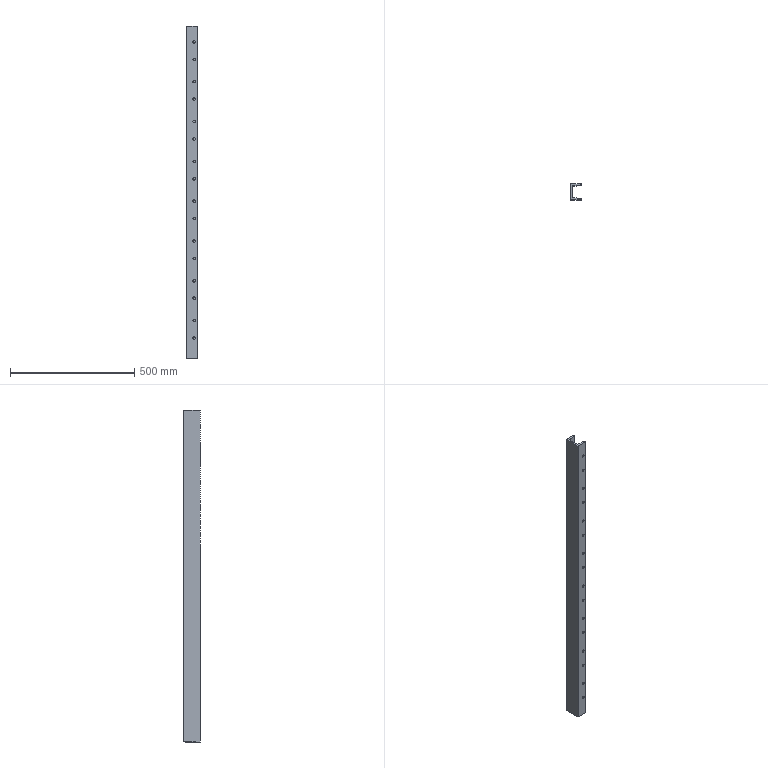Part | STEP file | DIN 1026-1 U 65 1785352380506 | 1 solid | 30 faces | box 42 x 65 x 1334 mm | volume 1196644 mm3 | cylinder 20 | plane 10 | commonest cylinder face diameters 10 x16 8 x2 15 x2
STEP:
#1=CARTESIAN_POINT('',(24.5,-32.5,1200.233));
#2=VERTEX_POINT('',#1);
#3=CARTESIAN_POINT('',(29.5,-32.5,1200.233));
#4=DIRECTION('',(0.,1.,0.));
#5=DIRECTION('',(1.,0.,0.));
#6=AXIS2_PLACEMENT_3D('',#3,#4,#5);
#7=CIRCLE('',#6,5.);
#8=EDGE_CURVE('',#2,#2,#7,.T.);
#9=ORIENTED_EDGE('',*,*,#8,.F.);
#10=CARTESIAN_POINT('',(24.5,-25.28,1200.233));
#11=VERTEX_POINT('',#10);
#12=CARTESIAN_POINT('',(24.5,-32.5,1200.233));
#13=DIRECTION('',(0.,1.,0.));
#14=VECTOR('',#13,5.);
#15=LINE('',#12,#14);
#16=EDGE_CURVE('',#2,#11,#15,.T.);
#17=ORIENTED_EDGE('',*,*,#16,.T.);
#18=CARTESIAN_POINT('',(29.5,-25.68,1200.233));
#19=DIRECTION('',(-0.07975,-0.9968,0.));
#20=DIRECTION('',(0.9968,-0.07975,0.));
#21=AXIS2_PLACEMENT_3D('',#18,#19,#20);
#22=ELLIPSE('',#21,5.016,5.);
#23=EDGE_CURVE('',#11,#11,#22,.T.);
#24=ORIENTED_EDGE('',*,*,#23,.F.);
#25=ORIENTED_EDGE('',*,*,#16,.F.);
#26=EDGE_LOOP('',(#9,#17,#24,#25));
#27=FACE_OUTER_BOUND('',#26,.T.);
#28=CARTESIAN_POINT('',(29.5,-32.5,1200.233));
#29=DIRECTION('',(0.,1.,0.));
#30=DIRECTION('',(1.,0.,0.));
#31=AXIS2_PLACEMENT_3D('',#28,#29,#30);
#32=CYLINDRICAL_SURFACE('',#31,5.);
#33=ADVANCED_FACE('',(#27),#32,.F.);
#34=CARTESIAN_POINT('',(24.5,-32.5,1270.233));
#35=VERTEX_POINT('',#34);
#36=CARTESIAN_POINT('',(29.5,-32.5,1270.233));
#37=DIRECTION('',(0.,1.,0.));
#38=DIRECTION('',(1.,0.,0.));
#39=AXIS2_PLACEMENT_3D('',#36,#37,#38);
#40=CIRCLE('',#39,5.);
#41=EDGE_CURVE('',#35,#35,#40,.T.);
#42=ORIENTED_EDGE('',*,*,#41,.F.);
#43=CARTESIAN_POINT('',(24.5,-25.28,1270.233));
#44=VERTEX_POINT('',#43);
#45=CARTESIAN_POINT('',(24.5,-32.5,1270.233));
#46=DIRECTION('',(0.,1.,0.));
#47=VECTOR('',#46,5.);
#48=LINE('',#45,#47);
#49=EDGE_CURVE('',#35,#44,#48,.T.);
#50=ORIENTED_EDGE('',*,*,#49,.T.);
#51=CARTESIAN_POINT('',(29.5,-25.68,1270.233));
#52=DIRECTION('',(-0.07975,-0.9968,0.));
#53=DIRECTION('',(0.9968,-0.07975,0.));
#54=AXIS2_PLACEMENT_3D('',#51,#52,#53);
#55=ELLIPSE('',#54,5.016,5.);
#56=EDGE_CURVE('',#44,#44,#55,.T.);
#57=ORIENTED_EDGE('',*,*,#56,.F.);
#58=ORIENTED_EDGE('',*,*,#49,.F.);
#59=EDGE_LOOP('',(#42,#50,#57,#58));
#60=FACE_OUTER_BOUND('',#59,.T.);
#61=CARTESIAN_POINT('',(29.5,-32.5,1270.233));
#62=DIRECTION('',(0.,1.,0.));
#63=DIRECTION('',(1.,0.,0.));
#64=AXIS2_PLACEMENT_3D('',#61,#62,#63);
#65=CYLINDRICAL_SURFACE('',#64,5.);
#66=ADVANCED_FACE('',(#60),#65,.F.);
#67=CARTESIAN_POINT('',(24.5,-32.5,1040.233));
#68=VERTEX_POINT('',#67);
#69=CARTESIAN_POINT('',(29.5,-32.5,1040.233));
#70=DIRECTION('',(0.,1.,0.));
#71=DIRECTION('',(1.,0.,0.));
#72=AXIS2_PLACEMENT_3D('',#69,#70,#71);
#73=CIRCLE('',#72,5.);
#74=EDGE_CURVE('',#68,#68,#73,.T.);
#75=ORIENTED_EDGE('',*,*,#74,.F.);
#76=CARTESIAN_POINT('',(24.5,-25.28,1040.233));
#77=VERTEX_POINT('',#76);
#78=CARTESIAN_POINT('',(24.5,-32.5,1040.233));
#79=DIRECTION('',(0.,1.,0.));
#80=VECTOR('',#79,5.);
#81=LINE('',#78,#80);
#82=EDGE_CURVE('',#68,#77,#81,.T.);
#83=ORIENTED_EDGE('',*,*,#82,.T.);
#84=CARTESIAN_POINT('',(29.5,-25.68,1040.233));
#85=DIRECTION('',(-0.07975,-0.9968,0.));
#86=DIRECTION('',(0.9968,-0.07975,0.));
#87=AXIS2_PLACEMENT_3D('',#84,#85,#86);
#88=ELLIPSE('',#87,5.016,5.);
#89=EDGE_CURVE('',#77,#77,#88,.T.);
#90=ORIENTED_EDGE('',*,*,#89,.F.);
#91=ORIENTED_EDGE('',*,*,#82,.F.);
#92=EDGE_LOOP('',(#75,#83,#90,#91));
#93=FACE_OUTER_BOUND('',#92,.T.);
#94=CARTESIAN_POINT('',(29.5,-32.5,1040.233));
#95=DIRECTION('',(0.,1.,0.));
#96=DIRECTION('',(1.,0.,0.));
#97=AXIS2_PLACEMENT_3D('',#94,#95,#96);
#98=CYLINDRICAL_SURFACE('',#97,5.);
#99=ADVANCED_FACE('',(#93),#98,.F.);
#100=CARTESIAN_POINT('',(24.5,-32.5,1110.233));
#101=VERTEX_POINT('',#100);
#102=CARTESIAN_POINT('',(29.5,-32.5,1110.233));
#103=DIRECTION('',(0.,1.,0.));
#104=DIRECTION('',(1.,0.,0.));
#105=AXIS2_PLACEMENT_3D('',#102,#103,#104);
#106=CIRCLE('',#105,5.);
#107=EDGE_CURVE('',#101,#101,#106,.T.);
#108=ORIENTED_EDGE('',*,*,#107,.F.);
#109=CARTESIAN_POINT('',(24.5,-25.28,1110.233));
#110=VERTEX_POINT('',#109);
#111=CARTESIAN_POINT('',(24.5,-32.5,1110.233));
#112=DIRECTION('',(0.,1.,0.));
#113=VECTOR('',#112,5.);
#114=LINE('',#111,#113);
#115=EDGE_CURVE('',#101,#110,#114,.T.);
#116=ORIENTED_EDGE('',*,*,#115,.T.);
#117=CARTESIAN_POINT('',(29.5,-25.68,1110.233));
#118=DIRECTION('',(-0.07975,-0.9968,0.));
#119=DIRECTION('',(0.9968,-0.07975,0.));
#120=AXIS2_PLACEMENT_3D('',#117,#118,#119);
#121=ELLIPSE('',#120,5.016,5.);
#122=EDGE_CURVE('',#110,#110,#121,.T.);
#123=ORIENTED_EDGE('',*,*,#122,.F.);
#124=ORIENTED_EDGE('',*,*,#115,.F.);
#125=EDGE_LOOP('',(#108,#116,#123,#124));
#126=FACE_OUTER_BOUND('',#125,.T.);
#127=CARTESIAN_POINT('',(29.5,-32.5,1110.233));
#128=DIRECTION('',(0.,1.,0.));
#129=DIRECTION('',(1.,0.,0.));
#130=AXIS2_PLACEMENT_3D('',#127,#128,#129);
#131=CYLINDRICAL_SURFACE('',#130,5.);
#132=ADVANCED_FACE('',(#126),#131,.F.);
#133=CARTESIAN_POINT('',(24.5,-32.5,880.233));
#134=VERTEX_POINT('',#133);
#135=CARTESIAN_POINT('',(29.5,-32.5,880.233));
#136=DIRECTION('',(0.,1.,0.));
#137=DIRECTION('',(1.,0.,0.));
#138=AXIS2_PLACEMENT_3D('',#135,#136,#137);
#139=CIRCLE('',#138,5.);
#140=EDGE_CURVE('',#134,#134,#139,.T.);
#141=ORIENTED_EDGE('',*,*,#140,.F.);
#142=CARTESIAN_POINT('',(24.5,-25.28,880.233));
#143=VERTEX_POINT('',#142);
#144=CARTESIAN_POINT('',(24.5,-32.5,880.233));
#145=DIRECTION('',(0.,1.,0.));
#146=VECTOR('',#145,5.);
#147=LINE('',#144,#146);
#148=EDGE_CURVE('',#134,#143,#147,.T.);
#149=ORIENTED_EDGE('',*,*,#148,.T.);
#150=CARTESIAN_POINT('',(29.5,-25.68,880.233));
#151=DIRECTION('',(-0.07975,-0.9968,0.));
#152=DIRECTION('',(0.9968,-0.07975,0.));
#153=AXIS2_PLACEMENT_3D('',#150,#151,#152);
#154=ELLIPSE('',#153,5.016,5.);
#155=EDGE_CURVE('',#143,#143,#154,.T.);
#156=ORIENTED_EDGE('',*,*,#155,.F.);
#157=ORIENTED_EDGE('',*,*,#148,.F.);
#158=EDGE_LOOP('',(#141,#149,#156,#157));
#159=FACE_OUTER_BOUND('',#158,.T.);
#160=CARTESIAN_POINT('',(29.5,-32.5,880.233));
#161=DIRECTION('',(0.,1.,0.));
#162=DIRECTION('',(1.,0.,0.));
#163=AXIS2_PLACEMENT_3D('',#160,#161,#162);
#164=CYLINDRICAL_SURFACE('',#163,5.);
#165=ADVANCED_FACE('',(#159),#164,.F.);
#166=CARTESIAN_POINT('',(24.5,-32.5,950.233));
#167=VERTEX_POINT('',#166);
#168=CARTESIAN_POINT('',(29.5,-32.5,950.233));
#169=DIRECTION('',(0.,1.,0.));
#170=DIRECTION('',(1.,0.,0.));
#171=AXIS2_PLACEMENT_3D('',#168,#169,#170);
#172=CIRCLE('',#171,5.);
#173=EDGE_CURVE('',#167,#167,#172,.T.);
#174=ORIENTED_EDGE('',*,*,#173,.F.);
#175=CARTESIAN_POINT('',(24.5,-25.28,950.233));
#176=VERTEX_POINT('',#175);
#177=CARTESIAN_POINT('',(24.5,-32.5,950.233));
#178=DIRECTION('',(0.,1.,0.));
#179=VECTOR('',#178,5.);
#180=LINE('',#177,#179);
#181=EDGE_CURVE('',#167,#176,#180,.T.);
#182=ORIENTED_EDGE('',*,*,#181,.T.);
#183=CARTESIAN_POINT('',(29.5,-25.68,950.233));
#184=DIRECTION('',(-0.07975,-0.9968,0.));
#185=DIRECTION('',(0.9968,-0.07975,0.));
#186=AXIS2_PLACEMENT_3D('',#183,#184,#185);
#187=ELLIPSE('',#186,5.016,5.);
#188=EDGE_CURVE('',#176,#176,#187,.T.);
#189=ORIENTED_EDGE('',*,*,#188,.F.);
#190=ORIENTED_EDGE('',*,*,#181,.F.);
#191=EDGE_LOOP('',(#174,#182,#189,#190));
#192=FACE_OUTER_BOUND('',#191,.T.);
#193=CARTESIAN_POINT('',(29.5,-32.5,950.233));
#194=DIRECTION('',(0.,1.,0.));
#195=DIRECTION('',(1.,0.,0.));
#196=AXIS2_PLACEMENT_3D('',#193,#194,#195);
#197=CYLINDRICAL_SURFACE('',#196,5.);
#198=ADVANCED_FACE('',(#192),#197,.F.);
#199=CARTESIAN_POINT('',(24.5,-32.5,720.233));
#200=VERTEX_POINT('',#199);
#201=CARTESIAN_POINT('',(29.5,-32.5,720.233));
#202=DIRECTION('',(0.,1.,0.));
#203=DIRECTION('',(1.,0.,0.));
#204=AXIS2_PLACEMENT_3D('',#201,#202,#203);
#205=CIRCLE('',#204,5.);
#206=EDGE_CURVE('',#200,#200,#205,.T.);
#207=ORIENTED_EDGE('',*,*,#206,.F.);
#208=CARTESIAN_POINT('',(24.5,-25.28,720.233));
#209=VERTEX_POINT('',#208);
#210=CARTESIAN_POINT('',(24.5,-32.5,720.233));
#211=DIRECTION('',(0.,1.,0.));
#212=VECTOR('',#211,5.);
#213=LINE('',#210,#212);
#214=EDGE_CURVE('',#200,#209,#213,.T.);
#215=ORIENTED_EDGE('',*,*,#214,.T.);
#216=CARTESIAN_POINT('',(29.5,-25.68,720.233));
#217=DIRECTION('',(-0.07975,-0.9968,0.));
#218=DIRECTION('',(0.9968,-0.07975,0.));
#219=AXIS2_PLACEMENT_3D('',#216,#217,#218);
#220=ELLIPSE('',#219,5.016,5.);
#221=EDGE_CURVE('',#209,#209,#220,.T.);
#222=ORIENTED_EDGE('',*,*,#221,.F.);
#223=ORIENTED_EDGE('',*,*,#214,.F.);
#224=EDGE_LOOP('',(#207,#215,#222,#223));
#225=FACE_OUTER_BOUND('',#224,.T.);
#226=CARTESIAN_POINT('',(29.5,-32.5,720.233));
#227=DIRECTION('',(0.,1.,0.));
#228=DIRECTION('',(1.,0.,0.));
#229=AXIS2_PLACEMENT_3D('',#226,#227,#228);
#230=CYLINDRICAL_SURFACE('',#229,5.);
#231=ADVANCED_FACE('',(#225),#230,.F.);
#232=CARTESIAN_POINT('',(24.5,-32.5,790.233));
#233=VERTEX_POINT('',#232);
#234=CARTESIAN_POINT('',(29.5,-32.5,790.233));
#235=DIRECTION('',(0.,1.,0.));
#236=DIRECTION('',(1.,0.,0.));
#237=AXIS2_PLACEMENT_3D('',#234,#235,#236);
#238=CIRCLE('',#237,5.);
#239=EDGE_CURVE('',#233,#233,#238,.T.);
#240=ORIENTED_EDGE('',*,*,#239,.F.);
#241=CARTESIAN_POINT('',(24.5,-25.28,790.233));
#242=VERTEX_POINT('',#241);
#243=CARTESIAN_POINT('',(24.5,-32.5,790.233));
#244=DIRECTION('',(0.,1.,0.));
#245=VECTOR('',#244,5.);
#246=LINE('',#243,#245);
#247=EDGE_CURVE('',#233,#242,#246,.T.);
#248=ORIENTED_EDGE('',*,*,#247,.T.);
#249=CARTESIAN_POINT('',(29.5,-25.68,790.233));
#250=DIRECTION('',(-0.07975,-0.9968,0.));
#251=DIRECTION('',(0.9968,-0.07975,0.));
#252=AXIS2_PLACEMENT_3D('',#249,#250,#251);
#253=ELLIPSE('',#252,5.016,5.);
#254=EDGE_CURVE('',#242,#242,#253,.T.);
#255=ORIENTED_EDGE('',*,*,#254,.F.);
#256=ORIENTED_EDGE('',*,*,#247,.F.);
#257=EDGE_LOOP('',(#240,#248,#255,#256));
#258=FACE_OUTER_BOUND('',#257,.T.);
#259=CARTESIAN_POINT('',(29.5,-32.5,790.233));
#260=DIRECTION('',(0.,1.,0.));
#261=DIRECTION('',(1.,0.,0.));
#262=AXIS2_PLACEMENT_3D('',#259,#260,#261);
#263=CYLINDRICAL_SURFACE('',#262,5.);
#264=ADVANCED_FACE('',(#258),#263,.F.);
#265=CARTESIAN_POINT('',(24.5,-32.5,560.233));
#266=VERTEX_POINT('',#265);
#267=CARTESIAN_POINT('',(29.5,-32.5,560.233));
#268=DIRECTION('',(0.,1.,0.));
#269=DIRECTION('',(1.,0.,0.));
#270=AXIS2_PLACEMENT_3D('',#267,#268,#269);
#271=CIRCLE('',#270,5.);
#272=EDGE_CURVE('',#266,#266,#271,.T.);
#273=ORIENTED_EDGE('',*,*,#272,.F.);
#274=CARTESIAN_POINT('',(24.5,-25.28,560.233));
#275=VERTEX_POINT('',#274);
#276=CARTESIAN_POINT('',(24.5,-32.5,560.233));
#277=DIRECTION('',(0.,1.,0.));
#278=VECTOR('',#277,5.);
#279=LINE('',#276,#278);
#280=EDGE_CURVE('',#266,#275,#279,.T.);
#281=ORIENTED_EDGE('',*,*,#280,.T.);
#282=CARTESIAN_POINT('',(29.5,-25.68,560.233));
#283=DIRECTION('',(-0.07975,-0.9968,0.));
#284=DIRECTION('',(0.9968,-0.07975,0.));
#285=AXIS2_PLACEMENT_3D('',#282,#283,#284);
#286=ELLIPSE('',#285,5.016,5.);
#287=EDGE_CURVE('',#275,#275,#286,.T.);
#288=ORIENTED_EDGE('',*,*,#287,.F.);
#289=ORIENTED_EDGE('',*,*,#280,.F.);
#290=EDGE_LOOP('',(#273,#281,#288,#289));
#291=FACE_OUTER_BOUND('',#290,.T.);
#292=CARTESIAN_POINT('',(29.5,-32.5,560.233));
#293=DIRECTION('',(0.,1.,0.));
#294=DIRECTION('',(1.,0.,0.));
#295=AXIS2_PLACEMENT_3D('',#292,#293,#294);
#296=CYLINDRICAL_SURFACE('',#295,5.);
#297=ADVANCED_FACE('',(#291),#296,.F.);
#298=CARTESIAN_POINT('',(24.5,-32.5,630.233));
#299=VERTEX_POINT('',#298);
#300=CARTESIAN_POINT('',(29.5,-32.5,630.233));
#301=DIRECTION('',(0.,1.,0.));
#302=DIRECTION('',(1.,0.,0.));
#303=AXIS2_PLACEMENT_3D('',#300,#301,#302);
#304=CIRCLE('',#303,5.);
#305=EDGE_CURVE('',#299,#299,#304,.T.);
#306=ORIENTED_EDGE('',*,*,#305,.F.);
#307=CARTESIAN_POINT('',(24.5,-25.28,630.233));
#308=VERTEX_POINT('',#307);
#309=CARTESIAN_POINT('',(24.5,-32.5,630.233));
#310=DIRECTION('',(0.,1.,0.));
#311=VECTOR('',#310,5.);
#312=LINE('',#309,#311);
#313=EDGE_CURVE('',#299,#308,#312,.T.);
#314=ORIENTED_EDGE('',*,*,#313,.T.);
#315=CARTESIAN_POINT('',(29.5,-25.68,630.233));
#316=DIRECTION('',(-0.07975,-0.9968,0.));
#317=DIRECTION('',(0.9968,-0.07975,0.));
#318=AXIS2_PLACEMENT_3D('',#315,#316,#317);
#319=ELLIPSE('',#318,5.016,5.);
#320=EDGE_CURVE('',#308,#308,#319,.T.);
#321=ORIENTED_EDGE('',*,*,#320,.F.);
#322=ORIENTED_EDGE('',*,*,#313,.F.);
#323=EDGE_LOOP('',(#306,#314,#321,#322));
#324=FACE_OUTER_BOUND('',#323,.T.);
#325=CARTESIAN_POINT('',(29.5,-32.5,630.233));
#326=DIRECTION('',(0.,1.,0.));
#327=DIRECTION('',(1.,0.,0.));
#328=AXIS2_PLACEMENT_3D('',#325,#326,#327);
#329=CYLINDRICAL_SURFACE('',#328,5.);
#330=ADVANCED_FACE('',(#324),#329,.F.);
#331=CARTESIAN_POINT('',(24.5,-32.5,400.233));
#332=VERTEX_POINT('',#331);
#333=CARTESIAN_POINT('',(29.5,-32.5,400.233));
#334=DIRECTION('',(0.,1.,0.));
#335=DIRECTION('',(1.,0.,0.));
#336=AXIS2_PLACEMENT_3D('',#333,#334,#335);
#337=CIRCLE('',#336,5.);
#338=EDGE_CURVE('',#332,#332,#337,.T.);
#339=ORIENTED_EDGE('',*,*,#338,.F.);
#340=CARTESIAN_POINT('',(24.5,-25.28,400.233));
#341=VERTEX_POINT('',#340);
#342=CARTESIAN_POINT('',(24.5,-32.5,400.233));
#343=DIRECTION('',(0.,1.,0.));
#344=VECTOR('',#343,5.);
#345=LINE('',#342,#344);
#346=EDGE_CURVE('',#332,#341,#345,.T.);
#347=ORIENTED_EDGE('',*,*,#346,.T.);
#348=CARTESIAN_POINT('',(29.5,-25.68,400.233));
#349=DIRECTION('',(-0.07975,-0.9968,0.));
#350=DIRECTION('',(0.9968,-0.07975,0.));
#351=AXIS2_PLACEMENT_3D('',#348,#349,#350);
#352=ELLIPSE('',#351,5.016,5.);
#353=EDGE_CURVE('',#341,#341,#352,.T.);
#354=ORIENTED_EDGE('',*,*,#353,.F.);
#355=ORIENTED_EDGE('',*,*,#346,.F.);
#356=EDGE_LOOP('',(#339,#347,#354,#355));
#357=FACE_OUTER_BOUND('',#356,.T.);
#358=CARTESIAN_POINT('',(29.5,-32.5,400.233));
#359=DIRECTION('',(0.,1.,0.));
#360=DIRECTION('',(1.,0.,0.));
#361=AXIS2_PLACEMENT_3D('',#358,#359,#360);
#362=CYLINDRICAL_SURFACE('',#361,5.);
#363=ADVANCED_FACE('',(#357),#362,.F.);
#364=CARTESIAN_POINT('',(24.5,-32.5,470.233));
#365=VERTEX_POINT('',#364);
#366=CARTESIAN_POINT('',(29.5,-32.5,470.233));
#367=DIRECTION('',(0.,1.,0.));
#368=DIRECTION('',(1.,0.,0.));
#369=AXIS2_PLACEMENT_3D('',#366,#367,#368);
#370=CIRCLE('',#369,5.);
#371=EDGE_CURVE('',#365,#365,#370,.T.);
#372=ORIENTED_EDGE('',*,*,#371,.F.);
#373=CARTESIAN_POINT('',(24.5,-25.28,470.233));
#374=VERTEX_POINT('',#373);
#375=CARTESIAN_POINT('',(24.5,-32.5,470.233));
#376=DIRECTION('',(0.,1.,0.));
#377=VECTOR('',#376,5.);
#378=LINE('',#375,#377);
#379=EDGE_CURVE('',#365,#374,#378,.T.);
#380=ORIENTED_EDGE('',*,*,#379,.T.);
#381=CARTESIAN_POINT('',(29.5,-25.68,470.233));
#382=DIRECTION('',(-0.07975,-0.9968,0.));
#383=DIRECTION('',(0.9968,-0.07975,0.));
#384=AXIS2_PLACEMENT_3D('',#381,#382,#383);
#385=ELLIPSE('',#384,5.016,5.);
#386=EDGE_CURVE('',#374,#374,#385,.T.);
#387=ORIENTED_EDGE('',*,*,#386,.F.);
#388=ORIENTED_EDGE('',*,*,#379,.F.);
#389=EDGE_LOOP('',(#372,#380,#387,#388));
#390=FACE_OUTER_BOUND('',#389,.T.);
#391=CARTESIAN_POINT('',(29.5,-32.5,470.233));
#392=DIRECTION('',(0.,1.,0.));
#393=DIRECTION('',(1.,0.,0.));
#394=AXIS2_PLACEMENT_3D('',#391,#392,#393);
#395=CYLINDRICAL_SURFACE('',#394,5.);
#396=ADVANCED_FACE('',(#390),#395,.F.);
#397=CARTESIAN_POINT('',(24.5,-32.5,240.233));
#398=VERTEX_POINT('',#397);
#399=CARTESIAN_POINT('',(29.5,-32.5,240.233));
#400=DIRECTION('',(0.,1.,0.));
#401=DIRECTION('',(1.,0.,0.));
#402=AXIS2_PLACEMENT_3D('',#399,#400,#401);
#403=CIRCLE('',#402,5.);
#404=EDGE_CURVE('',#398,#398,#403,.T.);
#405=ORIENTED_EDGE('',*,*,#404,.F.);
#406=CARTESIAN_POINT('',(24.5,-25.28,240.233));
#407=VERTEX_POINT('',#406);
#408=CARTESIAN_POINT('',(24.5,-32.5,240.233));
#409=DIRECTION('',(0.,1.,0.));
#410=VECTOR('',#409,5.);
#411=LINE('',#408,#410);
#412=EDGE_CURVE('',#398,#407,#411,.T.);
#413=ORIENTED_EDGE('',*,*,#412,.T.);
#414=CARTESIAN_POINT('',(29.5,-25.68,240.233));
#415=DIRECTION('',(-0.07975,-0.9968,0.));
#416=DIRECTION('',(0.9968,-0.07975,0.));
#417=AXIS2_PLACEMENT_3D('',#414,#415,#416);
#418=ELLIPSE('',#417,5.016,5.);
#419=EDGE_CURVE('',#407,#407,#418,.T.);
#420=ORIENTED_EDGE('',*,*,#419,.F.);
#421=ORIENTED_EDGE('',*,*,#412,.F.);
#422=EDGE_LOOP('',(#405,#413,#420,#421));
#423=FACE_OUTER_BOUND('',#422,.T.);
#424=CARTESIAN_POINT('',(29.5,-32.5,240.233));
#425=DIRECTION('',(0.,1.,0.));
#426=DIRECTION('',(1.,0.,0.));
#427=AXIS2_PLACEMENT_3D('',#424,#425,#426);
#428=CYLINDRICAL_SURFACE('',#427,5.);
#429=ADVANCED_FACE('',(#423),#428,.F.);
#430=CARTESIAN_POINT('',(24.5,-32.5,310.233));
#431=VERTEX_POINT('',#430);
#432=CARTESIAN_POINT('',(29.5,-32.5,310.233));
#433=DIRECTION('',(0.,1.,0.));
#434=DIRECTION('',(1.,0.,0.));
#435=AXIS2_PLACEMENT_3D('',#432,#433,#434);
#436=CIRCLE('',#435,5.);
#437=EDGE_CURVE('',#431,#431,#436,.T.);
#438=ORIENTED_EDGE('',*,*,#437,.F.);
#439=CARTESIAN_POINT('',(24.5,-25.28,310.233));
#440=VERTEX_POINT('',#439);
#441=CARTESIAN_POINT('',(24.5,-32.5,310.233));
#442=DIRECTION('',(0.,1.,0.));
#443=VECTOR('',#442,5.);
#444=LINE('',#441,#443);
#445=EDGE_CURVE('',#431,#440,#444,.T.);
#446=ORIENTED_EDGE('',*,*,#445,.T.);
#447=CARTESIAN_POINT('',(29.5,-25.68,310.233));
#448=DIRECTION('',(-0.07975,-0.9968,0.));
#449=DIRECTION('',(0.9968,-0.07975,0.));
#450=AXIS2_PLACEMENT_3D('',#447,#448,#449);
#451=ELLIPSE('',#450,5.016,5.);
#452=EDGE_CURVE('',#440,#440,#451,.T.);
#453=ORIENTED_EDGE('',*,*,#452,.F.);
#454=ORIENTED_EDGE('',*,*,#445,.F.);
#455=EDGE_LOOP('',(#438,#446,#453,#454));
#456=FACE_OUTER_BOUND('',#455,.T.);
#457=CARTESIAN_POINT('',(29.5,-32.5,310.233));
#458=DIRECTION('',(0.,1.,0.));
#459=DIRECTION('',(1.,0.,0.));
#460=AXIS2_PLACEMENT_3D('',#457,#458,#459);
#461=CYLINDRICAL_SURFACE('',#460,5.);
#462=ADVANCED_FACE('',(#456),#461,.F.);
#463=CARTESIAN_POINT('',(24.5,-32.5,80.233));
#464=VERTEX_POINT('',#463);
#465=CARTESIAN_POINT('',(29.5,-32.5,80.233));
#466=DIRECTION('',(0.,1.,0.));
#467=DIRECTION('',(1.,0.,0.));
#468=AXIS2_PLACEMENT_3D('',#465,#466,#467);
#469=CIRCLE('',#468,5.);
#470=EDGE_CURVE('',#464,#464,#469,.T.);
#471=ORIENTED_EDGE('',*,*,#470,.F.);
#472=CARTESIAN_POINT('',(24.5,-25.28,80.233));
#473=VERTEX_POINT('',#472);
#474=CARTESIAN_POINT('',(24.5,-32.5,80.233));
#475=DIRECTION('',(0.,1.,0.));
#476=VECTOR('',#475,5.);
#477=LINE('',#474,#476);
#478=EDGE_CURVE('',#464,#473,#477,.T.);
#479=ORIENTED_EDGE('',*,*,#478,.T.);
#480=CARTESIAN_POINT('',(29.5,-25.68,80.233));
#481=DIRECTION('',(-0.07975,-0.9968,0.));
#482=DIRECTION('',(0.9968,-0.07975,0.));
#483=AXIS2_PLACEMENT_3D('',#480,#481,#482);
#484=ELLIPSE('',#483,5.016,5.);
#485=EDGE_CURVE('',#473,#473,#484,.T.);
#486=ORIENTED_EDGE('',*,*,#485,.F.);
#487=ORIENTED_EDGE('',*,*,#478,.F.);
#488=EDGE_LOOP('',(#471,#479,#486,#487));
#489=FACE_OUTER_BOUND('',#488,.T.);
#490=CARTESIAN_POINT('',(29.5,-32.5,80.233));
#491=DIRECTION('',(0.,1.,0.));
#492=DIRECTION('',(1.,0.,0.));
#493=AXIS2_PLACEMENT_3D('',#490,#491,#492);
#494=CYLINDRICAL_SURFACE('',#493,5.);
#495=ADVANCED_FACE('',(#489),#494,.F.);
#496=CARTESIAN_POINT('',(24.5,-32.5,150.233));
#497=VERTEX_POINT('',#496);
#498=CARTESIAN_POINT('',(29.5,-32.5,150.233));
#499=DIRECTION('',(0.,1.,0.));
#500=DIRECTION('',(1.,0.,0.));
#501=AXIS2_PLACEMENT_3D('',#498,#499,#500);
#502=CIRCLE('',#501,5.);
#503=EDGE_CURVE('',#497,#497,#502,.T.);
#504=ORIENTED_EDGE('',*,*,#503,.F.);
#505=CARTESIAN_POINT('',(24.5,-25.28,150.233));
#506=VERTEX_POINT('',#505);
#507=CARTESIAN_POINT('',(24.5,-32.5,150.233));
#508=DIRECTION('',(0.,1.,0.));
#509=VECTOR('',#508,5.);
#510=LINE('',#507,#509);
#511=EDGE_CURVE('',#497,#506,#510,.T.);
#512=ORIENTED_EDGE('',*,*,#511,.T.);
#513=CARTESIAN_POINT('',(29.5,-25.68,150.233));
#514=DIRECTION('',(-0.07975,-0.9968,0.));
#515=DIRECTION('',(0.9968,-0.07975,0.));
#516=AXIS2_PLACEMENT_3D('',#513,#514,#515);
#517=ELLIPSE('',#516,5.016,5.);
#518=EDGE_CURVE('',#506,#506,#517,.T.);
#519=ORIENTED_EDGE('',*,*,#518,.F.);
#520=ORIENTED_EDGE('',*,*,#511,.F.);
#521=EDGE_LOOP('',(#504,#512,#519,#520));
#522=FACE_OUTER_BOUND('',#521,.T.);
#523=CARTESIAN_POINT('',(29.5,-32.5,150.233));
#524=DIRECTION('',(0.,1.,0.));
#525=DIRECTION('',(1.,0.,0.));
#526=AXIS2_PLACEMENT_3D('',#523,#524,#525);
#527=CYLINDRICAL_SURFACE('',#526,5.);
#528=ADVANCED_FACE('',(#522),#527,.F.);
#529=CARTESIAN_POINT('',(5.5,-16.836,1334.315));
#530=VERTEX_POINT('',#529);
#531=CARTESIAN_POINT('',(12.402,-24.312,1334.315));
#532=VERTEX_POINT('',#531);
#533=CARTESIAN_POINT('',(13.,-16.836,1334.315));
#534=DIRECTION('',(0.,0.,1.));
#535=DIRECTION('',(-1.,0.,0.));
#536=AXIS2_PLACEMENT_3D('',#533,#534,#535);
#537=CIRCLE('',#536,7.5);
#538=EDGE_CURVE('',#530,#532,#537,.T.);
#539=ORIENTED_EDGE('',*,*,#538,.T.);
#540=CARTESIAN_POINT('',(12.402,-24.312,0.));
#541=VERTEX_POINT('',#540);
#542=CARTESIAN_POINT('',(12.402,-24.312,0.));
#543=DIRECTION('',(0.,0.,1.));
#544=VECTOR('',#543,10.);
#545=LINE('',#542,#544);
#546=EDGE_CURVE('',#541,#532,#545,.T.);
#547=ORIENTED_EDGE('',*,*,#546,.F.);
#548=CARTESIAN_POINT('',(5.5,-16.836,0.));
#549=VERTEX_POINT('',#548);
#550=CARTESIAN_POINT('',(13.,-16.836,0.));
#551=DIRECTION('',(0.,0.,1.));
#552=DIRECTION('',(-1.,0.,0.));
#553=AXIS2_PLACEMENT_3D('',#550,#551,#552);
#554=CIRCLE('',#553,7.5);
#555=EDGE_CURVE('',#549,#541,#554,.T.);
#556=ORIENTED_EDGE('',*,*,#555,.F.);
#557=CARTESIAN_POINT('',(5.5,-16.836,0.));
#558=DIRECTION('',(0.,0.,1.));
#559=VECTOR('',#558,10.);
#560=LINE('',#557,#559);
#561=EDGE_CURVE('',#549,#530,#560,.T.);
#562=ORIENTED_EDGE('',*,*,#561,.T.);
#563=EDGE_LOOP('',(#539,#547,#556,#562));
#564=FACE_OUTER_BOUND('',#563,.T.);
#565=CARTESIAN_POINT('',(13.,-16.836,0.));
#566=DIRECTION('',(0.,0.,1.));
#567=DIRECTION('',(-1.,0.,0.));
#568=AXIS2_PLACEMENT_3D('',#565,#566,#567);
#569=CYLINDRICAL_SURFACE('',#568,7.5);
#570=ADVANCED_FACE('',(#564),#569,.F.);
#571=CARTESIAN_POINT('',(38.319,-26.386,1334.315));
#572=VERTEX_POINT('',#571);
#573=CARTESIAN_POINT('',(15.707,-24.577,1334.315));
#574=DIRECTION('',(0.9968,-0.07975,0.));
#575=VECTOR('',#574,10.);
#576=LINE('',#573,#575);
#577=EDGE_CURVE('',#532,#572,#576,.T.);
#578=ORIENTED_EDGE('',*,*,#577,.T.);
#579=CARTESIAN_POINT('',(38.319,-26.386,0.));
#580=VERTEX_POINT('',#579);
#581=CARTESIAN_POINT('',(38.319,-26.386,0.));
#582=DIRECTION('',(0.,0.,1.));
#583=VECTOR('',#582,10.);
#584=LINE('',#581,#583);
#585=EDGE_CURVE('',#580,#572,#584,.T.);
#586=ORIENTED_EDGE('',*,*,#585,.F.);
#587=CARTESIAN_POINT('',(15.707,-24.577,0.));
#588=DIRECTION('',(0.9968,-0.07975,0.));
#589=VECTOR('',#588,10.);
#590=LINE('',#587,#589);
#591=EDGE_CURVE('',#541,#580,#590,.T.);
#592=ORIENTED_EDGE('',*,*,#591,.F.);
#593=ORIENTED_EDGE('',*,*,#546,.T.);
#594=EDGE_LOOP('',(#578,#586,#592,#593));
#595=FACE_OUTER_BOUND('',#594,.T.);
#596=ORIENTED_EDGE('',*,*,#23,.T.);
#597=EDGE_LOOP('',(#596));
#598=FACE_BOUND('',#597,.T.);
#599=ORIENTED_EDGE('',*,*,#56,.T.);
#600=EDGE_LOOP('',(#599));
#601=FACE_BOUND('',#600,.T.);
#602=ORIENTED_EDGE('',*,*,#89,.T.);
#603=EDGE_LOOP('',(#602));
#604=FACE_BOUND('',#603,.T.);
#605=ORIENTED_EDGE('',*,*,#122,.T.);
#606=EDGE_LOOP('',(#605));
#607=FACE_BOUND('',#606,.T.);
#608=ORIENTED_EDGE('',*,*,#155,.T.);
#609=EDGE_LOOP('',(#608));
#610=FACE_BOUND('',#609,.T.);
#611=ORIENTED_EDGE('',*,*,#188,.T.);
#612=EDGE_LOOP('',(#611));
#613=FACE_BOUND('',#612,.T.);
#614=ORIENTED_EDGE('',*,*,#221,.T.);
#615=EDGE_LOOP('',(#614));
#616=FACE_BOUND('',#615,.T.);
#617=ORIENTED_EDGE('',*,*,#254,.T.);
#618=EDGE_LOOP('',(#617));
#619=FACE_BOUND('',#618,.T.);
#620=ORIENTED_EDGE('',*,*,#287,.T.);
#621=EDGE_LOOP('',(#620));
#622=FACE_BOUND('',#621,.T.);
#623=ORIENTED_EDGE('',*,*,#320,.T.);
#624=EDGE_LOOP('',(#623));
#625=FACE_BOUND('',#624,.T.);
#626=ORIENTED_EDGE('',*,*,#353,.T.);
#627=EDGE_LOOP('',(#626));
#628=FACE_BOUND('',#627,.T.);
#629=ORIENTED_EDGE('',*,*,#386,.T.);
#630=EDGE_LOOP('',(#629));
#631=FACE_BOUND('',#630,.T.);
#632=ORIENTED_EDGE('',*,*,#419,.T.);
#633=EDGE_LOOP('',(#632));
#634=FACE_BOUND('',#633,.T.);
#635=ORIENTED_EDGE('',*,*,#452,.T.);
#636=EDGE_LOOP('',(#635));
#637=FACE_BOUND('',#636,.T.);
#638=ORIENTED_EDGE('',*,*,#485,.T.);
#639=EDGE_LOOP('',(#638));
#640=FACE_BOUND('',#639,.T.);
#641=ORIENTED_EDGE('',*,*,#518,.T.);
#642=EDGE_LOOP('',(#641));
#643=FACE_BOUND('',#642,.T.);
#644=CARTESIAN_POINT('',(12.402,-24.312,0.));
#645=DIRECTION('',(0.07975,0.9968,0.));
#646=DIRECTION('',(0.,0.,1.));
#647=AXIS2_PLACEMENT_3D('',#644,#645,#646);
#648=PLANE('',#647);
#649=ADVANCED_FACE('',(#595,#598,#601,#604,#607,#610,#613,#616,#619,#622,#625,#628,#631,#634,#637,#640,#643),#648,.T.);
#650=CARTESIAN_POINT('',(42.,-30.373,1334.315));
#651=VERTEX_POINT('',#650);
#652=CARTESIAN_POINT('',(38.,-30.373,1334.315));
#653=DIRECTION('',(0.,0.,-1.));
#654=DIRECTION('',(-1.,0.,0.));
#655=AXIS2_PLACEMENT_3D('',#652,#653,#654);
#656=CIRCLE('',#655,4.);
#657=EDGE_CURVE('',#572,#651,#656,.T.);
#658=ORIENTED_EDGE('',*,*,#657,.T.);
#659=CARTESIAN_POINT('',(42.,-30.373,0.));
#660=VERTEX_POINT('',#659);
#661=CARTESIAN_POINT('',(42.,-30.373,0.));
#662=DIRECTION('',(0.,0.,1.));
#663=VECTOR('',#662,10.);
#664=LINE('',#661,#663);
#665=EDGE_CURVE('',#660,#651,#664,.T.);
#666=ORIENTED_EDGE('',*,*,#665,.F.);
#667=CARTESIAN_POINT('',(38.,-30.373,0.));
#668=DIRECTION('',(0.,0.,-1.));
#669=DIRECTION('',(-1.,0.,0.));
#670=AXIS2_PLACEMENT_3D('',#667,#668,#669);
#671=CIRCLE('',#670,4.);
#672=EDGE_CURVE('',#580,#660,#671,.T.);
#673=ORIENTED_EDGE('',*,*,#672,.F.);
#674=ORIENTED_EDGE('',*,*,#585,.T.);
#675=EDGE_LOOP('',(#658,#666,#673,#674));
#676=FACE_OUTER_BOUND('',#675,.T.);
#677=CARTESIAN_POINT('',(38.,-30.373,0.));
#678=DIRECTION('',(0.,0.,1.));
#679=DIRECTION('',(-1.,0.,0.));
#680=AXIS2_PLACEMENT_3D('',#677,#678,#679);
#681=CYLINDRICAL_SURFACE('',#680,4.);
#682=ADVANCED_FACE('',(#676),#681,.T.);
#683=CARTESIAN_POINT('',(42.,-32.5,1334.315));
#684=VERTEX_POINT('',#683);
#685=CARTESIAN_POINT('',(42.,-15.186,1334.315));
#686=DIRECTION('',(0.,-1.,0.));
#687=VECTOR('',#686,10.);
#688=LINE('',#685,#687);
#689=EDGE_CURVE('',#651,#684,#688,.T.);
#690=ORIENTED_EDGE('',*,*,#689,.T.);
#691=CARTESIAN_POINT('',(42.,-32.5,0.));
#692=VERTEX_POINT('',#691);
#693=CARTESIAN_POINT('',(42.,-32.5,0.));
#694=DIRECTION('',(0.,0.,1.));
#695=VECTOR('',#694,10.);
#696=LINE('',#693,#695);
#697=EDGE_CURVE('',#692,#684,#696,.T.);
#698=ORIENTED_EDGE('',*,*,#697,.F.);
#699=CARTESIAN_POINT('',(42.,-15.186,0.));
#700=DIRECTION('',(0.,-1.,0.));
#701=VECTOR('',#700,10.);
#702=LINE('',#699,#701);
#703=EDGE_CURVE('',#660,#692,#702,.T.);
#704=ORIENTED_EDGE('',*,*,#703,.F.);
#705=ORIENTED_EDGE('',*,*,#665,.T.);
#706=EDGE_LOOP('',(#690,#698,#704,#705));
#707=FACE_OUTER_BOUND('',#706,.T.);
#708=CARTESIAN_POINT('',(42.,-30.373,0.));
#709=DIRECTION('',(1.,0.,0.));
#710=DIRECTION('',(0.,0.,-1.));
#711=AXIS2_PLACEMENT_3D('',#708,#709,#710);
#712=PLANE('',#711);
#713=ADVANCED_FACE('',(#707),#712,.T.);
#714=CARTESIAN_POINT('',(0.,-32.5,1334.315));
#715=VERTEX_POINT('',#714);
#716=CARTESIAN_POINT('',(31.5,-32.5,1334.315));
#717=DIRECTION('',(-1.,0.,0.));
#718=VECTOR('',#717,10.);
#719=LINE('',#716,#718);
#720=EDGE_CURVE('',#684,#715,#719,.T.);
#721=ORIENTED_EDGE('',*,*,#720,.T.);
#722=CARTESIAN_POINT('',(0.,-32.5,0.));
#723=VERTEX_POINT('',#722);
#724=CARTESIAN_POINT('',(0.,-32.5,0.));
#725=DIRECTION('',(0.,0.,1.));
#726=VECTOR('',#725,10.);
#727=LINE('',#724,#726);
#728=EDGE_CURVE('',#723,#715,#727,.T.);
#729=ORIENTED_EDGE('',*,*,#728,.F.);
#730=CARTESIAN_POINT('',(31.5,-32.5,0.));
#731=DIRECTION('',(-1.,0.,0.));
#732=VECTOR('',#731,10.);
#733=LINE('',#730,#732);
#734=EDGE_CURVE('',#692,#723,#733,.T.);
#735=ORIENTED_EDGE('',*,*,#734,.F.);
#736=ORIENTED_EDGE('',*,*,#697,.T.);
#737=EDGE_LOOP('',(#721,#729,#735,#736));
#738=FACE_OUTER_BOUND('',#737,.T.);
#739=ORIENTED_EDGE('',*,*,#8,.T.);
#740=EDGE_LOOP('',(#739));
#741=FACE_BOUND('',#740,.T.);
#742=ORIENTED_EDGE('',*,*,#41,.T.);
#743=EDGE_LOOP('',(#742));
#744=FACE_BOUND('',#743,.T.);
#745=ORIENTED_EDGE('',*,*,#74,.T.);
#746=EDGE_LOOP('',(#745));
#747=FACE_BOUND('',#746,.T.);
#748=ORIENTED_EDGE('',*,*,#107,.T.);
#749=EDGE_LOOP('',(#748));
#750=FACE_BOUND('',#749,.T.);
#751=ORIENTED_EDGE('',*,*,#140,.T.);
#752=EDGE_LOOP('',(#751));
#753=FACE_BOUND('',#752,.T.);
#754=ORIENTED_EDGE('',*,*,#173,.T.);
#755=EDGE_LOOP('',(#754));
#756=FACE_BOUND('',#755,.T.);
#757=ORIENTED_EDGE('',*,*,#206,.T.);
#758=EDGE_LOOP('',(#757));
#759=FACE_BOUND('',#758,.T.);
#760=ORIENTED_EDGE('',*,*,#239,.T.);
#761=EDGE_LOOP('',(#760));
#762=FACE_BOUND('',#761,.T.);
#763=ORIENTED_EDGE('',*,*,#272,.T.);
#764=EDGE_LOOP('',(#763));
#765=FACE_BOUND('',#764,.T.);
#766=ORIENTED_EDGE('',*,*,#305,.T.);
#767=EDGE_LOOP('',(#766));
#768=FACE_BOUND('',#767,.T.);
#769=ORIENTED_EDGE('',*,*,#338,.T.);
#770=EDGE_LOOP('',(#769));
#771=FACE_BOUND('',#770,.T.);
#772=ORIENTED_EDGE('',*,*,#371,.T.);
#773=EDGE_LOOP('',(#772));
#774=FACE_BOUND('',#773,.T.);
#775=ORIENTED_EDGE('',*,*,#404,.T.);
#776=EDGE_LOOP('',(#775));
#777=FACE_BOUND('',#776,.T.);
#778=ORIENTED_EDGE('',*,*,#437,.T.);
#779=EDGE_LOOP('',(#778));
#780=FACE_BOUND('',#779,.T.);
#781=ORIENTED_EDGE('',*,*,#470,.T.);
#782=EDGE_LOOP('',(#781));
#783=FACE_BOUND('',#782,.T.);
#784=ORIENTED_EDGE('',*,*,#503,.T.);
#785=EDGE_LOOP('',(#784));
#786=FACE_BOUND('',#785,.T.);
#787=CARTESIAN_POINT('',(42.,-32.5,0.));
#788=DIRECTION('',(0.,-1.,0.));
#789=DIRECTION('',(0.,0.,-1.));
#790=AXIS2_PLACEMENT_3D('',#787,#788,#789);
#791=PLANE('',#790);
#792=ADVANCED_FACE('',(#738,#741,#744,#747,#750,#753,#756,#759,#762,#765,#768,#771,#774,#777,#780,#783,#786),#791,.T.);
#793=CARTESIAN_POINT('',(0.,32.5,1334.315));
#794=VERTEX_POINT('',#793);
#795=CARTESIAN_POINT('',(0.,0.,1334.315));
#796=DIRECTION('',(0.,1.,0.));
#797=VECTOR('',#796,10.);
#798=LINE('',#795,#797);
#799=EDGE_CURVE('',#715,#794,#798,.T.);
#800=ORIENTED_EDGE('',*,*,#799,.T.);
#801=CARTESIAN_POINT('',(0.,32.5,0.));
#802=VERTEX_POINT('',#801);
#803=CARTESIAN_POINT('',(0.,32.5,0.));
#804=DIRECTION('',(0.,0.,1.));
#805=VECTOR('',#804,10.);
#806=LINE('',#803,#805);
#807=EDGE_CURVE('',#802,#794,#806,.T.);
#808=ORIENTED_EDGE('',*,*,#807,.F.);
#809=CARTESIAN_POINT('',(0.,0.,0.));
#810=DIRECTION('',(0.,1.,0.));
#811=VECTOR('',#810,10.);
#812=LINE('',#809,#811);
#813=EDGE_CURVE('',#723,#802,#812,.T.);
#814=ORIENTED_EDGE('',*,*,#813,.F.);
#815=ORIENTED_EDGE('',*,*,#728,.T.);
#816=EDGE_LOOP('',(#800,#808,#814,#815));
#817=FACE_OUTER_BOUND('',#816,.T.);
#818=CARTESIAN_POINT('',(0.,0.,0.));
#819=DIRECTION('',(-1.,0.,0.));
#820=DIRECTION('',(0.,0.,1.));
#821=AXIS2_PLACEMENT_3D('',#818,#819,#820);
#822=PLANE('',#821);
#823=ADVANCED_FACE('',(#817),#822,.T.);
#824=CARTESIAN_POINT('',(42.,32.5,1334.315));
#825=VERTEX_POINT('',#824);
#826=CARTESIAN_POINT('',(10.5,32.5,1334.315));
#827=DIRECTION('',(1.,0.,0.));
#828=VECTOR('',#827,10.);
#829=LINE('',#826,#828);
#830=EDGE_CURVE('',#794,#825,#829,.T.);
#831=ORIENTED_EDGE('',*,*,#830,.T.);
#832=CARTESIAN_POINT('',(42.,32.5,0.));
#833=VERTEX_POINT('',#832);
#834=CARTESIAN_POINT('',(42.,32.5,0.));
#835=DIRECTION('',(0.,0.,1.));
#836=VECTOR('',#835,10.);
#837=LINE('',#834,#836);
#838=EDGE_CURVE('',#833,#825,#837,.T.);
#839=ORIENTED_EDGE('',*,*,#838,.F.);
#840=CARTESIAN_POINT('',(10.5,32.5,0.));
#841=DIRECTION('',(1.,0.,0.));
#842=VECTOR('',#841,10.);
#843=LINE('',#840,#842);
#844=EDGE_CURVE('',#802,#833,#843,.T.);
#845=ORIENTED_EDGE('',*,*,#844,.F.);
#846=ORIENTED_EDGE('',*,*,#807,.T.);
#847=EDGE_LOOP('',(#831,#839,#845,#846));
#848=FACE_OUTER_BOUND('',#847,.T.);
#849=CARTESIAN_POINT('',(0.,32.5,0.));
#850=DIRECTION('',(0.,1.,0.));
#851=DIRECTION('',(0.,0.,1.));
#852=AXIS2_PLACEMENT_3D('',#849,#850,#851);
#853=PLANE('',#852);
#854=ADVANCED_FACE('',(#848),#853,.T.);
#855=CARTESIAN_POINT('',(42.,30.373,1334.315));
#856=VERTEX_POINT('',#855);
#857=CARTESIAN_POINT('',(42.,16.25,1334.315));
#858=DIRECTION('',(0.,-1.,0.));
#859=VECTOR('',#858,10.);
#860=LINE('',#857,#859);
#861=EDGE_CURVE('',#825,#856,#860,.T.);
#862=ORIENTED_EDGE('',*,*,#861,.T.);
#863=CARTESIAN_POINT('',(42.,30.373,0.));
#864=VERTEX_POINT('',#863);
#865=CARTESIAN_POINT('',(42.,30.373,0.));
#866=DIRECTION('',(0.,0.,1.));
#867=VECTOR('',#866,10.);
#868=LINE('',#865,#867);
#869=EDGE_CURVE('',#864,#856,#868,.T.);
#870=ORIENTED_EDGE('',*,*,#869,.F.);
#871=CARTESIAN_POINT('',(42.,16.25,0.));
#872=DIRECTION('',(0.,-1.,0.));
#873=VECTOR('',#872,10.);
#874=LINE('',#871,#873);
#875=EDGE_CURVE('',#833,#864,#874,.T.);
#876=ORIENTED_EDGE('',*,*,#875,.F.);
#877=ORIENTED_EDGE('',*,*,#838,.T.);
#878=EDGE_LOOP('',(#862,#870,#876,#877));
#879=FACE_OUTER_BOUND('',#878,.T.);
#880=CARTESIAN_POINT('',(42.,32.5,0.));
#881=DIRECTION('',(1.,0.,0.));
#882=DIRECTION('',(0.,0.,-1.));
#883=AXIS2_PLACEMENT_3D('',#880,#881,#882);
#884=PLANE('',#883);
#885=ADVANCED_FACE('',(#879),#884,.T.);
#886=CARTESIAN_POINT('',(38.319,26.386,1334.315));
#887=VERTEX_POINT('',#886);
#888=CARTESIAN_POINT('',(38.,30.373,1334.315));
#889=DIRECTION('',(0.,0.,-1.));
#890=DIRECTION('',(-0.07975,0.9968,0.));
#891=AXIS2_PLACEMENT_3D('',#888,#889,#890);
#892=CIRCLE('',#891,4.);
#893=EDGE_CURVE('',#856,#887,#892,.T.);
#894=ORIENTED_EDGE('',*,*,#893,.T.);
#895=CARTESIAN_POINT('',(38.319,26.386,0.));
#896=VERTEX_POINT('',#895);
#897=CARTESIAN_POINT('',(38.319,26.386,0.));
#898=DIRECTION('',(0.,0.,1.));
#899=VECTOR('',#898,10.);
#900=LINE('',#897,#899);
#901=EDGE_CURVE('',#896,#887,#900,.T.);
#902=ORIENTED_EDGE('',*,*,#901,.F.);
#903=CARTESIAN_POINT('',(38.,30.373,0.));
#904=DIRECTION('',(0.,0.,-1.));
#905=DIRECTION('',(-0.07975,0.9968,0.));
#906=AXIS2_PLACEMENT_3D('',#903,#904,#905);
#907=CIRCLE('',#906,4.);
#908=EDGE_CURVE('',#864,#896,#907,.T.);
#909=ORIENTED_EDGE('',*,*,#908,.F.);
#910=ORIENTED_EDGE('',*,*,#869,.T.);
#911=EDGE_LOOP('',(#894,#902,#909,#910));
#912=FACE_OUTER_BOUND('',#911,.T.);
#913=CARTESIAN_POINT('',(38.,30.373,0.));
#914=DIRECTION('',(0.,0.,1.));
#915=DIRECTION('',(-0.07975,0.9968,0.));
#916=AXIS2_PLACEMENT_3D('',#913,#914,#915);
#917=CYLINDRICAL_SURFACE('',#916,4.);
#918=ADVANCED_FACE('',(#912),#917,.T.);
#919=CARTESIAN_POINT('',(12.402,24.312,1334.315));
#920=VERTEX_POINT('',#919);
#921=CARTESIAN_POINT('',(28.666,25.613,1334.315));
#922=DIRECTION('',(-0.9968,-0.07975,0.));
#923=VECTOR('',#922,10.);
#924=LINE('',#921,#923);
#925=EDGE_CURVE('',#887,#920,#924,.T.);
#926=ORIENTED_EDGE('',*,*,#925,.T.);
#927=CARTESIAN_POINT('',(12.402,24.312,0.));
#928=VERTEX_POINT('',#927);
#929=CARTESIAN_POINT('',(12.402,24.312,0.));
#930=DIRECTION('',(0.,0.,1.));
#931=VECTOR('',#930,10.);
#932=LINE('',#929,#931);
#933=EDGE_CURVE('',#928,#920,#932,.T.);
#934=ORIENTED_EDGE('',*,*,#933,.F.);
#935=CARTESIAN_POINT('',(28.666,25.613,0.));
#936=DIRECTION('',(-0.9968,-0.07975,0.));
#937=VECTOR('',#936,10.);
#938=LINE('',#935,#937);
#939=EDGE_CURVE('',#896,#928,#938,.T.);
#940=ORIENTED_EDGE('',*,*,#939,.F.);
#941=ORIENTED_EDGE('',*,*,#901,.T.);
#942=EDGE_LOOP('',(#926,#934,#940,#941));
#943=FACE_OUTER_BOUND('',#942,.T.);
#944=CARTESIAN_POINT('',(38.319,26.386,0.));
#945=DIRECTION('',(0.07975,-0.9968,0.));
#946=DIRECTION('',(0.,0.,-1.));
#947=AXIS2_PLACEMENT_3D('',#944,#945,#946);
#948=PLANE('',#947);
#949=ADVANCED_FACE('',(#943),#948,.T.);
#950=CARTESIAN_POINT('',(5.5,16.836,1334.315));
#951=VERTEX_POINT('',#950);
#952=CARTESIAN_POINT('',(13.,16.836,1334.315));
#953=DIRECTION('',(0.,0.,1.));
#954=DIRECTION('',(-0.07975,0.9968,0.));
#955=AXIS2_PLACEMENT_3D('',#952,#953,#954);
#956=CIRCLE('',#955,7.5);
#957=EDGE_CURVE('',#920,#951,#956,.T.);
#958=ORIENTED_EDGE('',*,*,#957,.T.);
#959=CARTESIAN_POINT('',(5.5,16.836,0.));
#960=VERTEX_POINT('',#959);
#961=CARTESIAN_POINT('',(5.5,16.836,0.));
#962=DIRECTION('',(0.,0.,1.));
#963=VECTOR('',#962,10.);
#964=LINE('',#961,#963);
#965=EDGE_CURVE('',#960,#951,#964,.T.);
#966=ORIENTED_EDGE('',*,*,#965,.F.);
#967=CARTESIAN_POINT('',(13.,16.836,0.));
#968=DIRECTION('',(0.,0.,1.));
#969=DIRECTION('',(-0.07975,0.9968,0.));
#970=AXIS2_PLACEMENT_3D('',#967,#968,#969);
#971=CIRCLE('',#970,7.5);
#972=EDGE_CURVE('',#928,#960,#971,.T.);
#973=ORIENTED_EDGE('',*,*,#972,.F.);
#974=ORIENTED_EDGE('',*,*,#933,.T.);
#975=EDGE_LOOP('',(#958,#966,#973,#974));
#976=FACE_OUTER_BOUND('',#975,.T.);
#977=CARTESIAN_POINT('',(13.,16.836,0.));
#978=DIRECTION('',(0.,0.,1.));
#979=DIRECTION('',(-0.07975,0.9968,0.));
#980=AXIS2_PLACEMENT_3D('',#977,#978,#979);
#981=CYLINDRICAL_SURFACE('',#980,7.5);
#982=ADVANCED_FACE('',(#976),#981,.F.);
#983=CARTESIAN_POINT('',(5.5,0.,1334.315));
#984=DIRECTION('',(0.,-1.,0.));
#985=VECTOR('',#984,10.);
#986=LINE('',#983,#985);
#987=EDGE_CURVE('',#951,#530,#986,.T.);
#988=ORIENTED_EDGE('',*,*,#987,.T.);
#989=ORIENTED_EDGE('',*,*,#561,.F.);
#990=CARTESIAN_POINT('',(5.5,0.,0.));
#991=DIRECTION('',(0.,-1.,0.));
#992=VECTOR('',#991,10.);
#993=LINE('',#990,#992);
#994=EDGE_CURVE('',#960,#549,#993,.T.);
#995=ORIENTED_EDGE('',*,*,#994,.F.);
#996=ORIENTED_EDGE('',*,*,#965,.T.);
#997=EDGE_LOOP('',(#988,#989,#995,#996));
#998=FACE_OUTER_BOUND('',#997,.T.);
#999=CARTESIAN_POINT('',(5.5,0.,0.));
#1000=DIRECTION('',(1.,0.,0.));
#1001=DIRECTION('',(0.,0.,-1.));
#1002=AXIS2_PLACEMENT_3D('',#999,#1000,#1001);
#1003=PLANE('',#1002);
#1004=ADVANCED_FACE('',(#998),#1003,.T.);
#1005=ORIENTED_EDGE('',*,*,#844,.T.);
#1006=ORIENTED_EDGE('',*,*,#875,.T.);
#1007=ORIENTED_EDGE('',*,*,#908,.T.);
#1008=ORIENTED_EDGE('',*,*,#939,.T.);
#1009=ORIENTED_EDGE('',*,*,#972,.T.);
#1010=ORIENTED_EDGE('',*,*,#994,.T.);
#1011=ORIENTED_EDGE('',*,*,#555,.T.);
#1012=ORIENTED_EDGE('',*,*,#591,.T.);
#1013=ORIENTED_EDGE('',*,*,#672,.T.);
#1014=ORIENTED_EDGE('',*,*,#703,.T.);
#1015=ORIENTED_EDGE('',*,*,#734,.T.);
#1016=ORIENTED_EDGE('',*,*,#813,.T.);
#1017=EDGE_LOOP('',(#1005,#1006,#1007,#1008,#1009,#1010,#1011,#1012,#1013,#1014,#1015,#1016));
#1018=FACE_OUTER_BOUND('',#1017,.T.);
#1019=CARTESIAN_POINT('',(21.,0.,0.));
#1020=DIRECTION('',(0.,0.,1.));
#1021=DIRECTION('',(1.,0.,0.));
#1022=AXIS2_PLACEMENT_3D('',#1019,#1020,#1021);
#1023=PLANE('',#1022);
#1024=ADVANCED_FACE('',(#1018),#1023,.F.);
#1025=ORIENTED_EDGE('',*,*,#830,.F.);
#1026=ORIENTED_EDGE('',*,*,#799,.F.);
#1027=ORIENTED_EDGE('',*,*,#720,.F.);
#1028=ORIENTED_EDGE('',*,*,#689,.F.);
#1029=ORIENTED_EDGE('',*,*,#657,.F.);
#1030=ORIENTED_EDGE('',*,*,#577,.F.);
#1031=ORIENTED_EDGE('',*,*,#538,.F.);
#1032=ORIENTED_EDGE('',*,*,#987,.F.);
#1033=ORIENTED_EDGE('',*,*,#957,.F.);
#1034=ORIENTED_EDGE('',*,*,#925,.F.);
#1035=ORIENTED_EDGE('',*,*,#893,.F.);
#1036=ORIENTED_EDGE('',*,*,#861,.F.);
#1037=EDGE_LOOP('',(#1025,#1026,#1027,#1028,#1029,#1030,#1031,#1032,#1033,#1034,#1035,#1036));
#1038=FACE_OUTER_BOUND('',#1037,.T.);
#1039=CARTESIAN_POINT('',(21.,0.,1334.315));
#1040=DIRECTION('',(0.,0.,1.));
#1041=DIRECTION('',(1.,0.,0.));
#1042=AXIS2_PLACEMENT_3D('',#1039,#1040,#1041);
#1043=PLANE('',#1042);
#1044=ADVANCED_FACE('',(#1038),#1043,.T.);
#1045=CLOSED_SHELL('',(#33,#66,#99,#132,#165,#198,#231,#264,#297,#330,#363,#396,#429,#462,#495,#528,#570,#649,#682,#713,#792,#823,#854,#885,#918,#949,#982,#1004,#1024,#1044));
#1046=MANIFOLD_SOLID_BREP('',#1045);
#1047=(LENGTH_UNIT()NAMED_UNIT(*)SI_UNIT(.MILLI.,.METRE.));
#1048=UNCERTAINTY_MEASURE_WITH_UNIT(LENGTH_MEASURE(0.01),#1047,'','');
#1049=(NAMED_UNIT(*)PLANE_ANGLE_UNIT()SI_UNIT($,.RADIAN.));
#1050=(NAMED_UNIT(*)SI_UNIT($,.STERADIAN.)SOLID_ANGLE_UNIT());
#1051=(GEOMETRIC_REPRESENTATION_CONTEXT(3)GLOBAL_UNCERTAINTY_ASSIGNED_CONTEXT((#1048))GLOBAL_UNIT_ASSIGNED_CONTEXT((#1047,#1049,#1050))REPRESENTATION_CONTEXT('',''));
#1052=ADVANCED_BREP_SHAPE_REPRESENTATION('',(#1046),#1051);